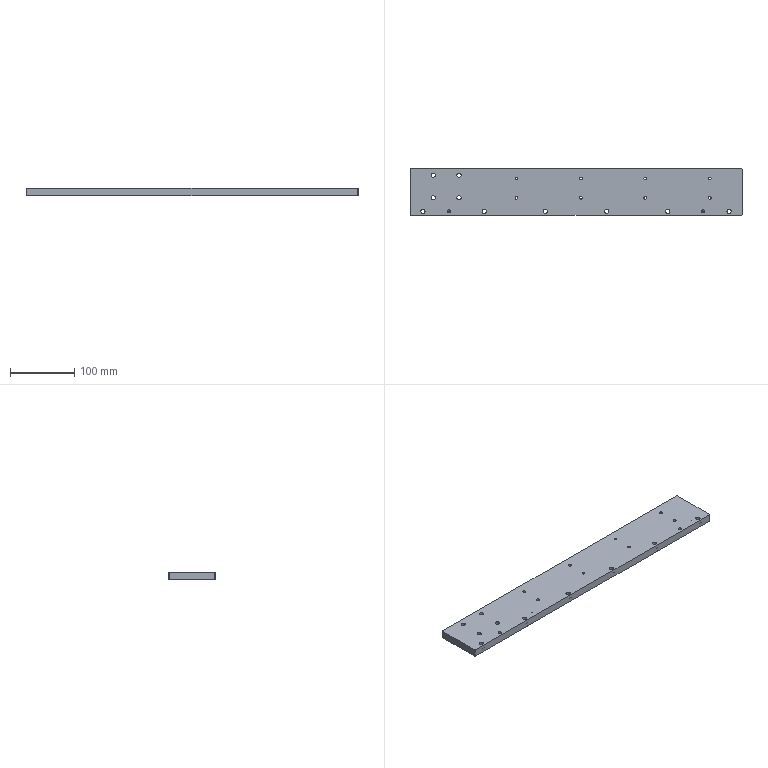Part | SolidWorks | features HoleWzd 5, Chamfer 1, Extrusion 1 | 1 solid | 92 faces | box 515 x 72 x 12 mm | volume 434783 mm3 | cylinder 64 | plane 20 | cone 8 | commonest cylinder face diameters 6.6 x20 11 x20 4.2 x16 5 x8